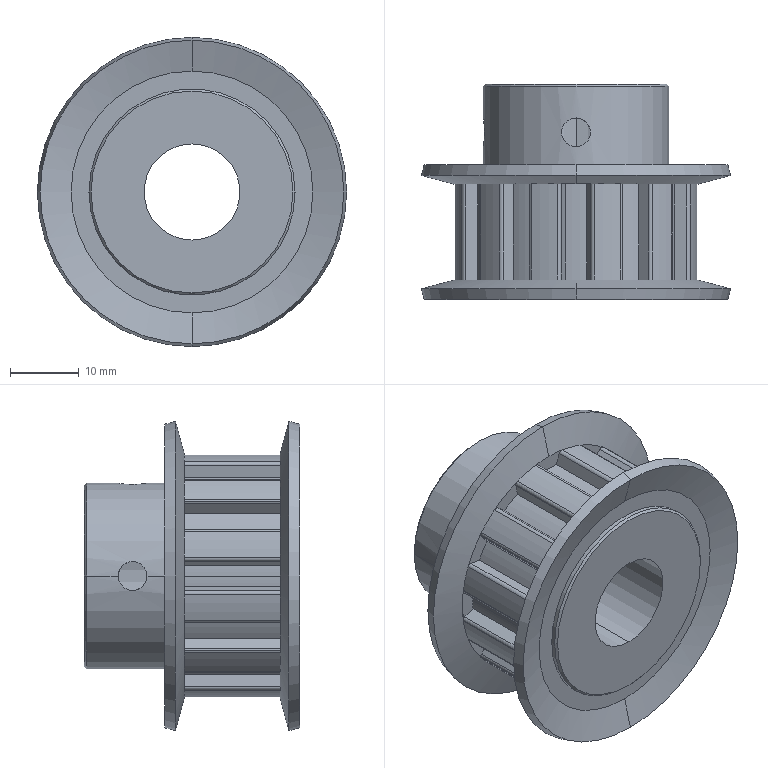Part | STEP file | 0243_Z_ATPP12L050-B-P14-KC90_2 | 1 solid | 140 faces | box 45 x 31.302 x 45 mm | volume 20799 mm3 | cylinder 69 | plane 53 | cone 18 | commonest cylinder face diameters 1.06 x30 31.36 x13 35.62 x12 4.2 x4 30 x4 1.72 x2